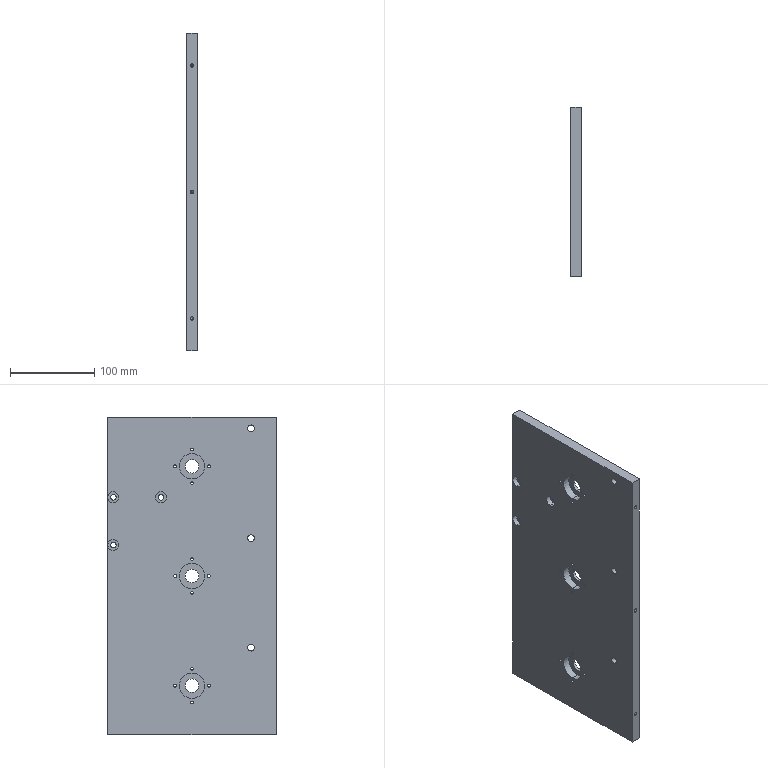Part | SolidWorks | features HoleWzd 1, MirrorStock 1 | 1 solid | 90 faces | box 12 x 200 x 376 mm | volume 873388 mm3 | cylinder 66 | cone 12 | plane 12 | commonest cylinder face diameters 3.3 x24 4.2 x12 6.6 x6 8 x6 13 x6 16 x6